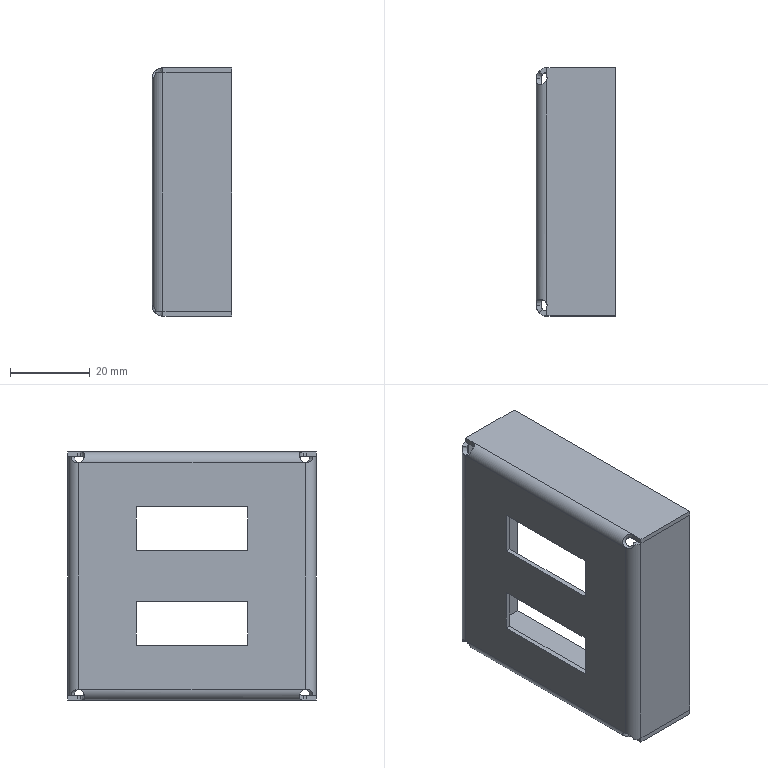Part | SolidWorks | features BaseBody 1 | 1 solid | 58 faces | box 20 x 62.4 x 62.4 mm | volume 9139 mm3 | plane 38 | cylinder 12 | spline 8 | commonest cylinder face diameters 3 x8 5.4 x4